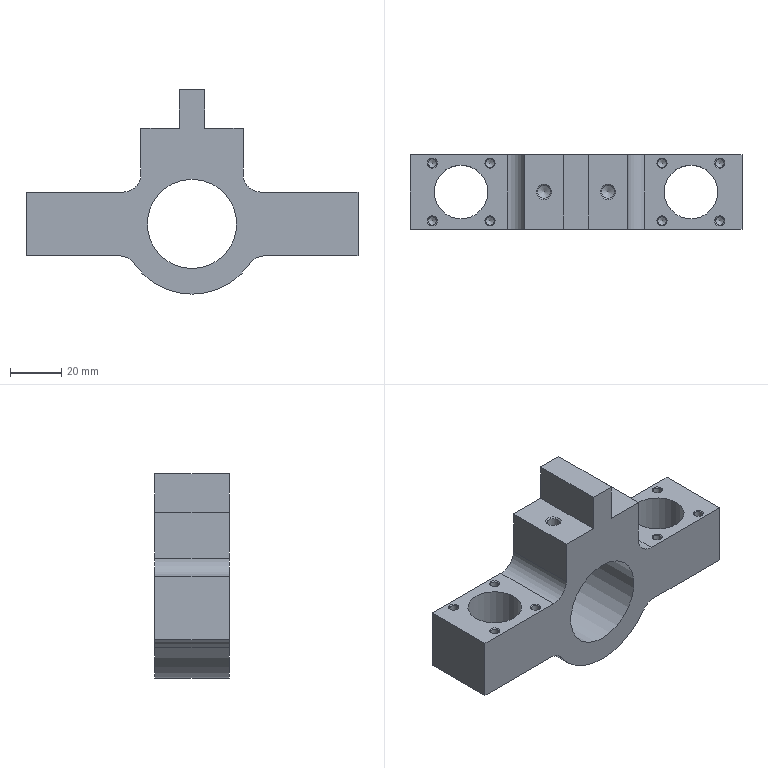Part | STEP file | YBQDJ-PD-12 | 1 solid | 53 faces | box 130 x 29.2 x 80 mm | volume 97793 mm3 | cone 20 | cylinder 18 | plane 15 | commonest cylinder face diameters 3.3 x8 14 x4 5 x2 21 x2 35 x1 55 x1